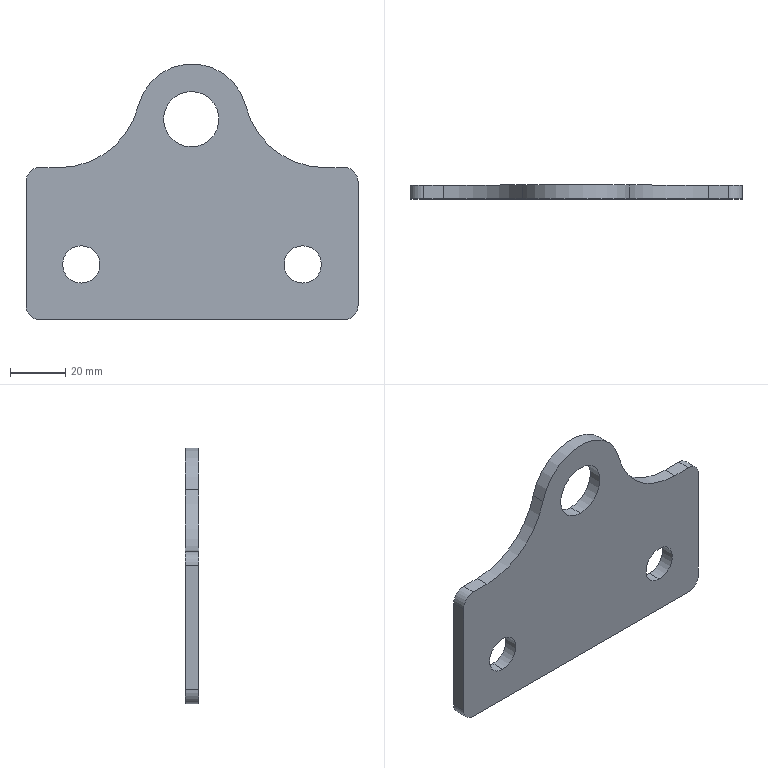Part | 1 solid | 20 faces | box 120 x 5 x 92.5 mm | volume 38056 mm3 | cylinder 13 | plane 7 | commonest cylinder face diameters 10 x4 13.5 x4 20 x2 58.94 x2 40 x1
STEP:
#1=CARTESIAN_POINT('',(40.,0.,-23.25));
#2=VERTEX_POINT('',#1);
#3=CARTESIAN_POINT('',(40.,0.,-36.75));
#4=VERTEX_POINT('',#3);
#5=CARTESIAN_POINT('',(40.,0.,-30.));
#6=DIRECTION('',(0.,-1.,0.));
#7=DIRECTION('',(0.,0.,-1.));
#8=AXIS2_PLACEMENT_3D('',#5,#6,#7);
#9=CIRCLE('',#8,6.75);
#10=EDGE_CURVE('',#2,#4,#9,.T.);
#11=ORIENTED_EDGE('',*,*,#10,.F.);
#12=CARTESIAN_POINT('',(40.,-5.,-23.25));
#13=VERTEX_POINT('',#12);
#14=CARTESIAN_POINT('',(40.,-5.,-23.25));
#15=DIRECTION('',(0.,-1.,0.));
#16=VECTOR('',#15,1000.);
#17=LINE('',#14,#16);
#18=EDGE_CURVE('',#2,#13,#17,.T.);
#19=ORIENTED_EDGE('',*,*,#18,.T.);
#20=CARTESIAN_POINT('',(40.,-5.,-36.75));
#21=VERTEX_POINT('',#20);
#22=CARTESIAN_POINT('',(40.,-5.,-30.));
#23=DIRECTION('',(0.,-1.,0.));
#24=DIRECTION('',(0.,0.,-1.));
#25=AXIS2_PLACEMENT_3D('',#22,#23,#24);
#26=CIRCLE('',#25,6.75);
#27=EDGE_CURVE('',#13,#21,#26,.T.);
#28=ORIENTED_EDGE('',*,*,#27,.T.);
#29=CARTESIAN_POINT('',(40.,-5.,-36.75));
#30=DIRECTION('',(0.,-1.,0.));
#31=VECTOR('',#30,1000.);
#32=LINE('',#29,#31);
#33=EDGE_CURVE('',#4,#21,#32,.T.);
#34=ORIENTED_EDGE('',*,*,#33,.F.);
#35=EDGE_LOOP('',(#11,#19,#28,#34));
#36=FACE_OUTER_BOUND('',#35,.T.);
#37=CARTESIAN_POINT('',(40.,-5.,-30.));
#38=DIRECTION('',(0.,-1.,0.));
#39=DIRECTION('',(0.,0.,-1.));
#40=AXIS2_PLACEMENT_3D('',#37,#38,#39);
#41=CYLINDRICAL_SURFACE('',#40,6.75);
#42=ADVANCED_FACE('',(#36),#41,.F.);
#43=CARTESIAN_POINT('',(-40.,0.,-23.25));
#44=VERTEX_POINT('',#43);
#45=CARTESIAN_POINT('',(-40.,0.,-36.75));
#46=VERTEX_POINT('',#45);
#47=CARTESIAN_POINT('',(-40.,0.,-30.));
#48=DIRECTION('',(0.,-1.,0.));
#49=DIRECTION('',(0.,0.,-1.));
#50=AXIS2_PLACEMENT_3D('',#47,#48,#49);
#51=CIRCLE('',#50,6.75);
#52=EDGE_CURVE('',#44,#46,#51,.T.);
#53=ORIENTED_EDGE('',*,*,#52,.F.);
#54=CARTESIAN_POINT('',(-40.,-5.,-23.25));
#55=VERTEX_POINT('',#54);
#56=CARTESIAN_POINT('',(-40.,-5.,-23.25));
#57=DIRECTION('',(0.,-1.,0.));
#58=VECTOR('',#57,1000.);
#59=LINE('',#56,#58);
#60=EDGE_CURVE('',#44,#55,#59,.T.);
#61=ORIENTED_EDGE('',*,*,#60,.T.);
#62=CARTESIAN_POINT('',(-40.,-5.,-36.75));
#63=VERTEX_POINT('',#62);
#64=CARTESIAN_POINT('',(-40.,-5.,-30.));
#65=DIRECTION('',(0.,-1.,0.));
#66=DIRECTION('',(0.,0.,-1.));
#67=AXIS2_PLACEMENT_3D('',#64,#65,#66);
#68=CIRCLE('',#67,6.75);
#69=EDGE_CURVE('',#55,#63,#68,.T.);
#70=ORIENTED_EDGE('',*,*,#69,.T.);
#71=CARTESIAN_POINT('',(-40.,-5.,-36.75));
#72=DIRECTION('',(0.,-1.,0.));
#73=VECTOR('',#72,1000.);
#74=LINE('',#71,#73);
#75=EDGE_CURVE('',#46,#63,#74,.T.);
#76=ORIENTED_EDGE('',*,*,#75,.F.);
#77=EDGE_LOOP('',(#53,#61,#70,#76));
#78=FACE_OUTER_BOUND('',#77,.T.);
#79=CARTESIAN_POINT('',(-40.,-5.,-30.));
#80=DIRECTION('',(0.,-1.,0.));
#81=DIRECTION('',(0.,0.,-1.));
#82=AXIS2_PLACEMENT_3D('',#79,#80,#81);
#83=CYLINDRICAL_SURFACE('',#82,6.75);
#84=ADVANCED_FACE('',(#78),#83,.F.);
#85=CARTESIAN_POINT('',(-0.25,-5.,32.5));
#86=VERTEX_POINT('',#85);
#87=CARTESIAN_POINT('',(-0.25,-5.,12.5));
#88=VERTEX_POINT('',#87);
#89=CARTESIAN_POINT('',(-0.25,-5.,22.5));
#90=DIRECTION('',(0.,-1.,0.));
#91=DIRECTION('',(0.,0.,-1.));
#92=AXIS2_PLACEMENT_3D('',#89,#90,#91);
#93=CIRCLE('',#92,10.);
#94=EDGE_CURVE('',#86,#88,#93,.T.);
#95=ORIENTED_EDGE('',*,*,#94,.T.);
#96=CARTESIAN_POINT('',(-0.25,0.,12.5));
#97=VERTEX_POINT('',#96);
#98=CARTESIAN_POINT('',(-0.25,-10.,12.5));
#99=DIRECTION('',(0.,1.,0.));
#100=VECTOR('',#99,1000.);
#101=LINE('',#98,#100);
#102=EDGE_CURVE('',#88,#97,#101,.T.);
#103=ORIENTED_EDGE('',*,*,#102,.T.);
#104=CARTESIAN_POINT('',(-0.25,0.,32.5));
#105=VERTEX_POINT('',#104);
#106=CARTESIAN_POINT('',(-0.25,0.,22.5));
#107=DIRECTION('',(0.,1.,0.));
#108=DIRECTION('',(0.,0.,1.));
#109=AXIS2_PLACEMENT_3D('',#106,#107,#108);
#110=CIRCLE('',#109,10.);
#111=EDGE_CURVE('',#97,#105,#110,.T.);
#112=ORIENTED_EDGE('',*,*,#111,.T.);
#113=CARTESIAN_POINT('',(-0.25,-10.,32.5));
#114=DIRECTION('',(0.,1.,0.));
#115=VECTOR('',#114,1000.);
#116=LINE('',#113,#115);
#117=EDGE_CURVE('',#86,#105,#116,.T.);
#118=ORIENTED_EDGE('',*,*,#117,.F.);
#119=EDGE_LOOP('',(#95,#103,#112,#118));
#120=FACE_OUTER_BOUND('',#119,.T.);
#121=CARTESIAN_POINT('',(-0.25,-10.,22.5));
#122=DIRECTION('',(0.,1.,0.));
#123=DIRECTION('',(0.,0.,1.));
#124=AXIS2_PLACEMENT_3D('',#121,#122,#123);
#125=CYLINDRICAL_SURFACE('',#124,10.);
#126=ADVANCED_FACE('',(#120),#125,.F.);
#127=CARTESIAN_POINT('',(40.,-5.,-30.));
#128=DIRECTION('',(0.,-1.,0.));
#129=DIRECTION('',(0.,0.,-1.));
#130=AXIS2_PLACEMENT_3D('',#127,#128,#129);
#131=CIRCLE('',#130,6.75);
#132=EDGE_CURVE('',#21,#13,#131,.T.);
#133=ORIENTED_EDGE('',*,*,#132,.F.);
#134=ORIENTED_EDGE('',*,*,#27,.F.);
#135=EDGE_LOOP('',(#133,#134));
#136=FACE_BOUND('',#135,.T.);
#137=CARTESIAN_POINT('',(-40.,-5.,-30.));
#138=DIRECTION('',(0.,-1.,0.));
#139=DIRECTION('',(0.,0.,-1.));
#140=AXIS2_PLACEMENT_3D('',#137,#138,#139);
#141=CIRCLE('',#140,6.75);
#142=EDGE_CURVE('',#63,#55,#141,.T.);
#143=ORIENTED_EDGE('',*,*,#142,.F.);
#144=ORIENTED_EDGE('',*,*,#69,.F.);
#145=EDGE_LOOP('',(#143,#144));
#146=FACE_BOUND('',#145,.T.);
#147=ORIENTED_EDGE('',*,*,#94,.F.);
#148=CARTESIAN_POINT('',(-0.25,-5.,22.5));
#149=DIRECTION('',(0.,-1.,0.));
#150=DIRECTION('',(0.,0.,-1.));
#151=AXIS2_PLACEMENT_3D('',#148,#149,#150);
#152=CIRCLE('',#151,10.);
#153=EDGE_CURVE('',#88,#86,#152,.T.);
#154=ORIENTED_EDGE('',*,*,#153,.F.);
#155=EDGE_LOOP('',(#147,#154));
#156=FACE_BOUND('',#155,.T.);
#157=CARTESIAN_POINT('',(-60.,-5.,-45.));
#158=VERTEX_POINT('',#157);
#159=CARTESIAN_POINT('',(-60.,-5.,0.));
#160=VERTEX_POINT('',#159);
#161=CARTESIAN_POINT('',(-60.,-5.,50.));
#162=DIRECTION('',(0.,0.,1.));
#163=VECTOR('',#162,1000.);
#164=LINE('',#161,#163);
#165=EDGE_CURVE('',#158,#160,#164,.T.);
#166=ORIENTED_EDGE('',*,*,#165,.F.);
#167=CARTESIAN_POINT('',(-55.,-5.,-50.));
#168=VERTEX_POINT('',#167);
#169=CARTESIAN_POINT('',(-55.,-5.,-45.));
#170=DIRECTION('',(0.,-1.,0.));
#171=DIRECTION('',(0.,0.,-1.));
#172=AXIS2_PLACEMENT_3D('',#169,#170,#171);
#173=CIRCLE('',#172,5.);
#174=EDGE_CURVE('',#158,#168,#173,.T.);
#175=ORIENTED_EDGE('',*,*,#174,.T.);
#176=CARTESIAN_POINT('',(55.,-5.,-50.));
#177=VERTEX_POINT('',#176);
#178=CARTESIAN_POINT('',(-60.,-5.,-50.));
#179=DIRECTION('',(-1.,0.,0.));
#180=VECTOR('',#179,1000.);
#181=LINE('',#178,#180);
#182=EDGE_CURVE('',#177,#168,#181,.T.);
#183=ORIENTED_EDGE('',*,*,#182,.F.);
#184=CARTESIAN_POINT('',(60.,-5.,-45.));
#185=VERTEX_POINT('',#184);
#186=CARTESIAN_POINT('',(55.,-5.,-45.));
#187=DIRECTION('',(0.,-1.,0.));
#188=DIRECTION('',(0.,0.,-1.));
#189=AXIS2_PLACEMENT_3D('',#186,#187,#188);
#190=CIRCLE('',#189,5.);
#191=EDGE_CURVE('',#177,#185,#190,.T.);
#192=ORIENTED_EDGE('',*,*,#191,.T.);
#193=CARTESIAN_POINT('',(60.,-5.,0.));
#194=VERTEX_POINT('',#193);
#195=CARTESIAN_POINT('',(60.,-5.,50.));
#196=DIRECTION('',(0.,0.,-1.));
#197=VECTOR('',#196,1000.);
#198=LINE('',#195,#197);
#199=EDGE_CURVE('',#194,#185,#198,.T.);
#200=ORIENTED_EDGE('',*,*,#199,.F.);
#201=CARTESIAN_POINT('',(55.,-5.,5.));
#202=VERTEX_POINT('',#201);
#203=CARTESIAN_POINT('',(55.,-5.,0.));
#204=DIRECTION('',(0.,-1.,0.));
#205=DIRECTION('',(0.,0.,-1.));
#206=AXIS2_PLACEMENT_3D('',#203,#204,#205);
#207=CIRCLE('',#206,5.);
#208=EDGE_CURVE('',#194,#202,#207,.T.);
#209=ORIENTED_EDGE('',*,*,#208,.T.);
#210=CARTESIAN_POINT('',(48.,-5.,5.));
#211=VERTEX_POINT('',#210);
#212=CARTESIAN_POINT('',(60.,-5.,5.));
#213=DIRECTION('',(1.,0.,0.));
#214=VECTOR('',#213,1000.);
#215=LINE('',#212,#214);
#216=EDGE_CURVE('',#211,#202,#215,.T.);
#217=ORIENTED_EDGE('',*,*,#216,.F.);
#218=CARTESIAN_POINT('',(19.406,-5.,27.339));
#219=VERTEX_POINT('',#218);
#220=CARTESIAN_POINT('',(48.,-5.,34.47));
#221=DIRECTION('',(0.,-1.,0.));
#222=DIRECTION('',(0.,0.,-1.));
#223=AXIS2_PLACEMENT_3D('',#220,#221,#222);
#224=CIRCLE('',#223,29.47);
#225=EDGE_CURVE('',#219,#211,#224,.T.);
#226=ORIENTED_EDGE('',*,*,#225,.F.);
#227=CARTESIAN_POINT('',(-19.406,-5.,27.339));
#228=VERTEX_POINT('',#227);
#229=CARTESIAN_POINT('',(0.,-5.,22.5));
#230=DIRECTION('',(0.,1.,0.));
#231=DIRECTION('',(0.,0.,-1.));
#232=AXIS2_PLACEMENT_3D('',#229,#230,#231);
#233=CIRCLE('',#232,20.);
#234=EDGE_CURVE('',#228,#219,#233,.T.);
#235=ORIENTED_EDGE('',*,*,#234,.F.);
#236=CARTESIAN_POINT('',(-48.,-5.,5.));
#237=VERTEX_POINT('',#236);
#238=CARTESIAN_POINT('',(-48.,-5.,34.47));
#239=DIRECTION('',(0.,-1.,0.));
#240=DIRECTION('',(0.,0.,1.));
#241=AXIS2_PLACEMENT_3D('',#238,#239,#240);
#242=CIRCLE('',#241,29.47);
#243=EDGE_CURVE('',#237,#228,#242,.T.);
#244=ORIENTED_EDGE('',*,*,#243,.F.);
#245=CARTESIAN_POINT('',(-55.,-5.,5.));
#246=VERTEX_POINT('',#245);
#247=CARTESIAN_POINT('',(-48.,-5.,5.));
#248=DIRECTION('',(1.,0.,0.));
#249=VECTOR('',#248,1000.);
#250=LINE('',#247,#249);
#251=EDGE_CURVE('',#246,#237,#250,.T.);
#252=ORIENTED_EDGE('',*,*,#251,.F.);
#253=CARTESIAN_POINT('',(-55.,-5.,0.));
#254=DIRECTION('',(0.,-1.,0.));
#255=DIRECTION('',(0.,0.,-1.));
#256=AXIS2_PLACEMENT_3D('',#253,#254,#255);
#257=CIRCLE('',#256,5.);
#258=EDGE_CURVE('',#246,#160,#257,.T.);
#259=ORIENTED_EDGE('',*,*,#258,.T.);
#260=EDGE_LOOP('',(#166,#175,#183,#192,#200,#209,#217,#226,#235,#244,#252,#259));
#261=FACE_OUTER_BOUND('',#260,.T.);
#262=CARTESIAN_POINT('',(0.,-5.,0.));
#263=DIRECTION('',(0.,-1.,0.));
#264=DIRECTION('',(0.,0.,-1.));
#265=AXIS2_PLACEMENT_3D('',#262,#263,#264);
#266=PLANE('',#265);
#267=ADVANCED_FACE('',(#136,#146,#156,#261),#266,.T.);
#268=CARTESIAN_POINT('',(40.,0.,-30.));
#269=DIRECTION('',(0.,-1.,0.));
#270=DIRECTION('',(0.,0.,-1.));
#271=AXIS2_PLACEMENT_3D('',#268,#269,#270);
#272=CIRCLE('',#271,6.75);
#273=EDGE_CURVE('',#4,#2,#272,.T.);
#274=ORIENTED_EDGE('',*,*,#273,.T.);
#275=ORIENTED_EDGE('',*,*,#10,.T.);
#276=EDGE_LOOP('',(#274,#275));
#277=FACE_BOUND('',#276,.T.);
#278=CARTESIAN_POINT('',(-40.,0.,-30.));
#279=DIRECTION('',(0.,-1.,0.));
#280=DIRECTION('',(0.,0.,-1.));
#281=AXIS2_PLACEMENT_3D('',#278,#279,#280);
#282=CIRCLE('',#281,6.75);
#283=EDGE_CURVE('',#46,#44,#282,.T.);
#284=ORIENTED_EDGE('',*,*,#283,.T.);
#285=ORIENTED_EDGE('',*,*,#52,.T.);
#286=EDGE_LOOP('',(#284,#285));
#287=FACE_BOUND('',#286,.T.);
#288=CARTESIAN_POINT('',(-0.25,0.,22.5));
#289=DIRECTION('',(0.,1.,0.));
#290=DIRECTION('',(0.,0.,1.));
#291=AXIS2_PLACEMENT_3D('',#288,#289,#290);
#292=CIRCLE('',#291,10.);
#293=EDGE_CURVE('',#105,#97,#292,.T.);
#294=ORIENTED_EDGE('',*,*,#293,.F.);
#295=ORIENTED_EDGE('',*,*,#111,.F.);
#296=EDGE_LOOP('',(#294,#295));
#297=FACE_BOUND('',#296,.T.);
#298=CARTESIAN_POINT('',(55.,0.,-50.));
#299=VERTEX_POINT('',#298);
#300=CARTESIAN_POINT('',(-55.,0.,-50.));
#301=VERTEX_POINT('',#300);
#302=CARTESIAN_POINT('',(-60.,0.,-50.));
#303=DIRECTION('',(-1.,0.,0.));
#304=VECTOR('',#303,1000.);
#305=LINE('',#302,#304);
#306=EDGE_CURVE('',#299,#301,#305,.T.);
#307=ORIENTED_EDGE('',*,*,#306,.T.);
#308=CARTESIAN_POINT('',(-60.,0.,-45.));
#309=VERTEX_POINT('',#308);
#310=CARTESIAN_POINT('',(-55.,0.,-45.));
#311=DIRECTION('',(0.,1.,0.));
#312=DIRECTION('',(0.,0.,-1.));
#313=AXIS2_PLACEMENT_3D('',#310,#311,#312);
#314=CIRCLE('',#313,5.);
#315=EDGE_CURVE('',#301,#309,#314,.T.);
#316=ORIENTED_EDGE('',*,*,#315,.T.);
#317=CARTESIAN_POINT('',(-60.,0.,0.));
#318=VERTEX_POINT('',#317);
#319=CARTESIAN_POINT('',(-60.,0.,50.));
#320=DIRECTION('',(0.,0.,1.));
#321=VECTOR('',#320,1000.);
#322=LINE('',#319,#321);
#323=EDGE_CURVE('',#309,#318,#322,.T.);
#324=ORIENTED_EDGE('',*,*,#323,.T.);
#325=CARTESIAN_POINT('',(-55.,0.,5.));
#326=VERTEX_POINT('',#325);
#327=CARTESIAN_POINT('',(-55.,0.,0.));
#328=DIRECTION('',(0.,1.,0.));
#329=DIRECTION('',(0.,0.,-1.));
#330=AXIS2_PLACEMENT_3D('',#327,#328,#329);
#331=CIRCLE('',#330,5.);
#332=EDGE_CURVE('',#318,#326,#331,.T.);
#333=ORIENTED_EDGE('',*,*,#332,.T.);
#334=CARTESIAN_POINT('',(-48.,0.,5.));
#335=VERTEX_POINT('',#334);
#336=CARTESIAN_POINT('',(-48.,0.,5.));
#337=DIRECTION('',(1.,0.,0.));
#338=VECTOR('',#337,1000.);
#339=LINE('',#336,#338);
#340=EDGE_CURVE('',#326,#335,#339,.T.);
#341=ORIENTED_EDGE('',*,*,#340,.T.);
#342=CARTESIAN_POINT('',(-19.406,0.,27.339));
#343=VERTEX_POINT('',#342);
#344=CARTESIAN_POINT('',(-48.,0.,34.47));
#345=DIRECTION('',(0.,-1.,0.));
#346=DIRECTION('',(0.,0.,1.));
#347=AXIS2_PLACEMENT_3D('',#344,#345,#346);
#348=CIRCLE('',#347,29.47);
#349=EDGE_CURVE('',#335,#343,#348,.T.);
#350=ORIENTED_EDGE('',*,*,#349,.T.);
#351=CARTESIAN_POINT('',(19.406,0.,27.339));
#352=VERTEX_POINT('',#351);
#353=CARTESIAN_POINT('',(0.,0.,22.5));
#354=DIRECTION('',(0.,1.,0.));
#355=DIRECTION('',(0.,0.,-1.));
#356=AXIS2_PLACEMENT_3D('',#353,#354,#355);
#357=CIRCLE('',#356,20.);
#358=EDGE_CURVE('',#343,#352,#357,.T.);
#359=ORIENTED_EDGE('',*,*,#358,.T.);
#360=CARTESIAN_POINT('',(48.,0.,5.));
#361=VERTEX_POINT('',#360);
#362=CARTESIAN_POINT('',(48.,0.,34.47));
#363=DIRECTION('',(0.,-1.,0.));
#364=DIRECTION('',(0.,0.,-1.));
#365=AXIS2_PLACEMENT_3D('',#362,#363,#364);
#366=CIRCLE('',#365,29.47);
#367=EDGE_CURVE('',#352,#361,#366,.T.);
#368=ORIENTED_EDGE('',*,*,#367,.T.);
#369=CARTESIAN_POINT('',(55.,0.,5.));
#370=VERTEX_POINT('',#369);
#371=CARTESIAN_POINT('',(60.,0.,5.));
#372=DIRECTION('',(1.,0.,0.));
#373=VECTOR('',#372,1000.);
#374=LINE('',#371,#373);
#375=EDGE_CURVE('',#361,#370,#374,.T.);
#376=ORIENTED_EDGE('',*,*,#375,.T.);
#377=CARTESIAN_POINT('',(60.,0.,0.));
#378=VERTEX_POINT('',#377);
#379=CARTESIAN_POINT('',(55.,0.,0.));
#380=DIRECTION('',(0.,1.,0.));
#381=DIRECTION('',(0.,0.,-1.));
#382=AXIS2_PLACEMENT_3D('',#379,#380,#381);
#383=CIRCLE('',#382,5.);
#384=EDGE_CURVE('',#370,#378,#383,.T.);
#385=ORIENTED_EDGE('',*,*,#384,.T.);
#386=CARTESIAN_POINT('',(60.,0.,-45.));
#387=VERTEX_POINT('',#386);
#388=CARTESIAN_POINT('',(60.,0.,50.));
#389=DIRECTION('',(0.,0.,-1.));
#390=VECTOR('',#389,1000.);
#391=LINE('',#388,#390);
#392=EDGE_CURVE('',#378,#387,#391,.T.);
#393=ORIENTED_EDGE('',*,*,#392,.T.);
#394=CARTESIAN_POINT('',(55.,0.,-45.));
#395=DIRECTION('',(0.,1.,0.));
#396=DIRECTION('',(0.,0.,-1.));
#397=AXIS2_PLACEMENT_3D('',#394,#395,#396);
#398=CIRCLE('',#397,5.);
#399=EDGE_CURVE('',#387,#299,#398,.T.);
#400=ORIENTED_EDGE('',*,*,#399,.T.);
#401=EDGE_LOOP('',(#307,#316,#324,#333,#341,#350,#359,#368,#376,#385,#393,#400));
#402=FACE_OUTER_BOUND('',#401,.T.);
#403=CARTESIAN_POINT('',(0.,0.,0.));
#404=DIRECTION('',(0.,-1.,0.));
#405=DIRECTION('',(0.,0.,-1.));
#406=AXIS2_PLACEMENT_3D('',#403,#404,#405);
#407=PLANE('',#406);
#408=ADVANCED_FACE('',(#277,#287,#297,#402),#407,.F.);
#409=ORIENTED_EDGE('',*,*,#199,.T.);
#410=CARTESIAN_POINT('',(60.,-5.,-45.));
#411=DIRECTION('',(0.,1.,0.));
#412=VECTOR('',#411,1000.);
#413=LINE('',#410,#412);
#414=EDGE_CURVE('',#185,#387,#413,.T.);
#415=ORIENTED_EDGE('',*,*,#414,.T.);
#416=ORIENTED_EDGE('',*,*,#392,.F.);
#417=CARTESIAN_POINT('',(60.,-5.,0.));
#418=DIRECTION('',(0.,-1.,0.));
#419=VECTOR('',#418,1000.);
#420=LINE('',#417,#419);
#421=EDGE_CURVE('',#378,#194,#420,.T.);
#422=ORIENTED_EDGE('',*,*,#421,.T.);
#423=EDGE_LOOP('',(#409,#415,#416,#422));
#424=FACE_OUTER_BOUND('',#423,.T.);
#425=CARTESIAN_POINT('',(60.,-5.,50.));
#426=DIRECTION('',(1.,0.,0.));
#427=DIRECTION('',(0.,0.,-1.));
#428=AXIS2_PLACEMENT_3D('',#425,#426,#427);
#429=PLANE('',#428);
#430=ADVANCED_FACE('',(#424),#429,.T.);
#431=ORIENTED_EDGE('',*,*,#323,.F.);
#432=CARTESIAN_POINT('',(-60.,-5.,-45.));
#433=DIRECTION('',(0.,-1.,0.));
#434=VECTOR('',#433,1000.);
#435=LINE('',#432,#434);
#436=EDGE_CURVE('',#309,#158,#435,.T.);
#437=ORIENTED_EDGE('',*,*,#436,.T.);
#438=ORIENTED_EDGE('',*,*,#165,.T.);
#439=CARTESIAN_POINT('',(-60.,0.,0.));
#440=DIRECTION('',(0.,1.,0.));
#441=VECTOR('',#440,1000.);
#442=LINE('',#439,#441);
#443=EDGE_CURVE('',#160,#318,#442,.T.);
#444=ORIENTED_EDGE('',*,*,#443,.T.);
#445=EDGE_LOOP('',(#431,#437,#438,#444));
#446=FACE_OUTER_BOUND('',#445,.T.);
#447=CARTESIAN_POINT('',(-60.,-5.,50.));
#448=DIRECTION('',(-1.,0.,0.));
#449=DIRECTION('',(0.,0.,1.));
#450=AXIS2_PLACEMENT_3D('',#447,#448,#449);
#451=PLANE('',#450);
#452=ADVANCED_FACE('',(#446),#451,.T.);
#453=ORIENTED_EDGE('',*,*,#182,.T.);
#454=CARTESIAN_POINT('',(-55.,-5.,-50.));
#455=DIRECTION('',(0.,1.,0.));
#456=VECTOR('',#455,1000.);
#457=LINE('',#454,#456);
#458=EDGE_CURVE('',#168,#301,#457,.T.);
#459=ORIENTED_EDGE('',*,*,#458,.T.);
#460=ORIENTED_EDGE('',*,*,#306,.F.);
#461=CARTESIAN_POINT('',(55.,-5.,-50.));
#462=DIRECTION('',(0.,-1.,0.));
#463=VECTOR('',#462,1000.);
#464=LINE('',#461,#463);
#465=EDGE_CURVE('',#299,#177,#464,.T.);
#466=ORIENTED_EDGE('',*,*,#465,.T.);
#467=EDGE_LOOP('',(#453,#459,#460,#466));
#468=FACE_OUTER_BOUND('',#467,.T.);
#469=CARTESIAN_POINT('',(-60.,-5.,-50.));
#470=DIRECTION('',(0.,0.,-1.));
#471=DIRECTION('',(-1.,0.,0.));
#472=AXIS2_PLACEMENT_3D('',#469,#470,#471);
#473=PLANE('',#472);
#474=ADVANCED_FACE('',(#468),#473,.T.);
#475=ORIENTED_EDGE('',*,*,#102,.F.);
#476=ORIENTED_EDGE('',*,*,#153,.T.);
#477=ORIENTED_EDGE('',*,*,#117,.T.);
#478=ORIENTED_EDGE('',*,*,#293,.T.);
#479=EDGE_LOOP('',(#475,#476,#477,#478));
#480=FACE_OUTER_BOUND('',#479,.T.);
#481=CARTESIAN_POINT('',(-0.25,-10.,22.5));
#482=DIRECTION('',(0.,1.,0.));
#483=DIRECTION('',(0.,0.,1.));
#484=AXIS2_PLACEMENT_3D('',#481,#482,#483);
#485=CYLINDRICAL_SURFACE('',#484,10.);
#486=ADVANCED_FACE('',(#480),#485,.F.);
#487=ORIENTED_EDGE('',*,*,#243,.T.);
#488=CARTESIAN_POINT('',(-19.406,0.,27.339));
#489=DIRECTION('',(0.,-1.,0.));
#490=VECTOR('',#489,1000.);
#491=LINE('',#488,#490);
#492=EDGE_CURVE('',#343,#228,#491,.T.);
#493=ORIENTED_EDGE('',*,*,#492,.F.);
#494=ORIENTED_EDGE('',*,*,#349,.F.);
#495=CARTESIAN_POINT('',(-48.,0.,5.));
#496=DIRECTION('',(0.,-1.,0.));
#497=VECTOR('',#496,1000.);
#498=LINE('',#495,#497);
#499=EDGE_CURVE('',#335,#237,#498,.T.);
#500=ORIENTED_EDGE('',*,*,#499,.T.);
#501=EDGE_LOOP('',(#487,#493,#494,#500));
#502=FACE_OUTER_BOUND('',#501,.T.);
#503=CARTESIAN_POINT('',(-48.,0.,34.47));
#504=DIRECTION('',(0.,-1.,0.));
#505=DIRECTION('',(0.,0.,-1.));
#506=AXIS2_PLACEMENT_3D('',#503,#504,#505);
#507=CYLINDRICAL_SURFACE('',#506,29.47);
#508=ADVANCED_FACE('',(#502),#507,.F.);
#509=ORIENTED_EDGE('',*,*,#340,.F.);
#510=CARTESIAN_POINT('',(-55.,-5.,5.));
#511=DIRECTION('',(0.,-1.,0.));
#512=VECTOR('',#511,1000.);
#513=LINE('',#510,#512);
#514=EDGE_CURVE('',#326,#246,#513,.T.);
#515=ORIENTED_EDGE('',*,*,#514,.T.);
#516=ORIENTED_EDGE('',*,*,#251,.T.);
#517=ORIENTED_EDGE('',*,*,#499,.F.);
#518=EDGE_LOOP('',(#509,#515,#516,#517));
#519=FACE_OUTER_BOUND('',#518,.T.);
#520=CARTESIAN_POINT('',(-48.,0.,5.));
#521=DIRECTION('',(0.,0.,-1.));
#522=DIRECTION('',(-1.,0.,0.));
#523=AXIS2_PLACEMENT_3D('',#520,#521,#522);
#524=PLANE('',#523);
#525=ADVANCED_FACE('',(#519),#524,.F.);
#526=ORIENTED_EDGE('',*,*,#216,.T.);
#527=CARTESIAN_POINT('',(55.,0.,5.));
#528=DIRECTION('',(0.,1.,0.));
#529=VECTOR('',#528,1000.);
#530=LINE('',#527,#529);
#531=EDGE_CURVE('',#202,#370,#530,.T.);
#532=ORIENTED_EDGE('',*,*,#531,.T.);
#533=ORIENTED_EDGE('',*,*,#375,.F.);
#534=CARTESIAN_POINT('',(48.,0.,5.));
#535=DIRECTION('',(0.,-1.,0.));
#536=VECTOR('',#535,1000.);
#537=LINE('',#534,#536);
#538=EDGE_CURVE('',#361,#211,#537,.T.);
#539=ORIENTED_EDGE('',*,*,#538,.T.);
#540=EDGE_LOOP('',(#526,#532,#533,#539));
#541=FACE_OUTER_BOUND('',#540,.T.);
#542=CARTESIAN_POINT('',(60.,0.,5.));
#543=DIRECTION('',(0.,0.,-1.));
#544=DIRECTION('',(-1.,0.,0.));
#545=AXIS2_PLACEMENT_3D('',#542,#543,#544);
#546=PLANE('',#545);
#547=ADVANCED_FACE('',(#541),#546,.F.);
#548=ORIENTED_EDGE('',*,*,#225,.T.);
#549=ORIENTED_EDGE('',*,*,#538,.F.);
#550=ORIENTED_EDGE('',*,*,#367,.F.);
#551=CARTESIAN_POINT('',(19.406,0.,27.339));
#552=DIRECTION('',(0.,-1.,0.));
#553=VECTOR('',#552,1000.);
#554=LINE('',#551,#553);
#555=EDGE_CURVE('',#352,#219,#554,.T.);
#556=ORIENTED_EDGE('',*,*,#555,.T.);
#557=EDGE_LOOP('',(#548,#549,#550,#556));
#558=FACE_OUTER_BOUND('',#557,.T.);
#559=CARTESIAN_POINT('',(48.,0.,34.47));
#560=DIRECTION('',(0.,-1.,0.));
#561=DIRECTION('',(0.,0.,-1.));
#562=AXIS2_PLACEMENT_3D('',#559,#560,#561);
#563=CYLINDRICAL_SURFACE('',#562,29.47);
#564=ADVANCED_FACE('',(#558),#563,.F.);
#565=ORIENTED_EDGE('',*,*,#234,.T.);
#566=ORIENTED_EDGE('',*,*,#555,.F.);
#567=ORIENTED_EDGE('',*,*,#358,.F.);
#568=ORIENTED_EDGE('',*,*,#492,.T.);
#569=EDGE_LOOP('',(#565,#566,#567,#568));
#570=FACE_OUTER_BOUND('',#569,.T.);
#571=CARTESIAN_POINT('',(0.,0.,22.5));
#572=DIRECTION('',(0.,-1.,0.));
#573=DIRECTION('',(0.,0.,-1.));
#574=AXIS2_PLACEMENT_3D('',#571,#572,#573);
#575=CYLINDRICAL_SURFACE('',#574,20.);
#576=ADVANCED_FACE('',(#570),#575,.T.);
#577=ORIENTED_EDGE('',*,*,#174,.F.);
#578=ORIENTED_EDGE('',*,*,#436,.F.);
#579=ORIENTED_EDGE('',*,*,#315,.F.);
#580=ORIENTED_EDGE('',*,*,#458,.F.);
#581=EDGE_LOOP('',(#577,#578,#579,#580));
#582=FACE_OUTER_BOUND('',#581,.T.);
#583=CARTESIAN_POINT('',(-55.,-5.,-45.));
#584=DIRECTION('',(0.,1.,0.));
#585=DIRECTION('',(0.,0.,1.));
#586=AXIS2_PLACEMENT_3D('',#583,#584,#585);
#587=CYLINDRICAL_SURFACE('',#586,5.);
#588=ADVANCED_FACE('',(#582),#587,.T.);
#589=ORIENTED_EDGE('',*,*,#332,.F.);
#590=ORIENTED_EDGE('',*,*,#443,.F.);
#591=ORIENTED_EDGE('',*,*,#258,.F.);
#592=ORIENTED_EDGE('',*,*,#514,.F.);
#593=EDGE_LOOP('',(#589,#590,#591,#592));
#594=FACE_OUTER_BOUND('',#593,.T.);
#595=CARTESIAN_POINT('',(-55.,0.,0.));
#596=DIRECTION('',(0.,1.,0.));
#597=DIRECTION('',(0.,0.,1.));
#598=AXIS2_PLACEMENT_3D('',#595,#596,#597);
#599=CYLINDRICAL_SURFACE('',#598,5.);
#600=ADVANCED_FACE('',(#594),#599,.T.);
#601=ORIENTED_EDGE('',*,*,#191,.F.);
#602=ORIENTED_EDGE('',*,*,#465,.F.);
#603=ORIENTED_EDGE('',*,*,#399,.F.);
#604=ORIENTED_EDGE('',*,*,#414,.F.);
#605=EDGE_LOOP('',(#601,#602,#603,#604));
#606=FACE_OUTER_BOUND('',#605,.T.);
#607=CARTESIAN_POINT('',(55.,-5.,-45.));
#608=DIRECTION('',(0.,1.,0.));
#609=DIRECTION('',(0.,0.,1.));
#610=AXIS2_PLACEMENT_3D('',#607,#608,#609);
#611=CYLINDRICAL_SURFACE('',#610,5.);
#612=ADVANCED_FACE('',(#606),#611,.T.);
#613=ORIENTED_EDGE('',*,*,#384,.F.);
#614=ORIENTED_EDGE('',*,*,#531,.F.);
#615=ORIENTED_EDGE('',*,*,#208,.F.);
#616=ORIENTED_EDGE('',*,*,#421,.F.);
#617=EDGE_LOOP('',(#613,#614,#615,#616));
#618=FACE_OUTER_BOUND('',#617,.T.);
#619=CARTESIAN_POINT('',(55.,-5.,0.));
#620=DIRECTION('',(0.,1.,0.));
#621=DIRECTION('',(0.,0.,1.));
#622=AXIS2_PLACEMENT_3D('',#619,#620,#621);
#623=CYLINDRICAL_SURFACE('',#622,5.);
#624=ADVANCED_FACE('',(#618),#623,.T.);
#625=ORIENTED_EDGE('',*,*,#60,.F.);
#626=ORIENTED_EDGE('',*,*,#283,.F.);
#627=ORIENTED_EDGE('',*,*,#75,.T.);
#628=ORIENTED_EDGE('',*,*,#142,.T.);
#629=EDGE_LOOP('',(#625,#626,#627,#628));
#630=FACE_OUTER_BOUND('',#629,.T.);
#631=CARTESIAN_POINT('',(-40.,-5.,-30.));
#632=DIRECTION('',(0.,-1.,0.));
#633=DIRECTION('',(0.,0.,-1.));
#634=AXIS2_PLACEMENT_3D('',#631,#632,#633);
#635=CYLINDRICAL_SURFACE('',#634,6.75);
#636=ADVANCED_FACE('',(#630),#635,.F.);
#637=ORIENTED_EDGE('',*,*,#18,.F.);
#638=ORIENTED_EDGE('',*,*,#273,.F.);
#639=ORIENTED_EDGE('',*,*,#33,.T.);
#640=ORIENTED_EDGE('',*,*,#132,.T.);
#641=EDGE_LOOP('',(#637,#638,#639,#640));
#642=FACE_OUTER_BOUND('',#641,.T.);
#643=CARTESIAN_POINT('',(40.,-5.,-30.));
#644=DIRECTION('',(0.,-1.,0.));
#645=DIRECTION('',(0.,0.,-1.));
#646=AXIS2_PLACEMENT_3D('',#643,#644,#645);
#647=CYLINDRICAL_SURFACE('',#646,6.75);
#648=ADVANCED_FACE('',(#642),#647,.F.);
#649=CLOSED_SHELL('',(#42,#84,#126,#267,#408,#430,#452,#474,#486,#508,#525,#547,#564,#576,#588,#600,#612,#624,#636,#648));
#650=MANIFOLD_SOLID_BREP('',#649);
#651=CARTESIAN_POINT('',(0.,0.,0.));
#652=DIRECTION('',(0.,0.,1.));
#653=DIRECTION('',(1.,0.,0.));
#654=AXIS2_PLACEMENT_3D('',#651,#652,#653);
#655=(LENGTH_UNIT()NAMED_UNIT(*)SI_UNIT(.MILLI.,.METRE.));
#656=UNCERTAINTY_MEASURE_WITH_UNIT(LENGTH_MEASURE(0.00001),#655,'','');
#657=(NAMED_UNIT(*)PLANE_ANGLE_UNIT()SI_UNIT($,.RADIAN.));
#658=(NAMED_UNIT(*)SI_UNIT($,.STERADIAN.)SOLID_ANGLE_UNIT());
#659=(GEOMETRIC_REPRESENTATION_CONTEXT(3)GLOBAL_UNCERTAINTY_ASSIGNED_CONTEXT((#656))GLOBAL_UNIT_ASSIGNED_CONTEXT((#655,#657,#658))REPRESENTATION_CONTEXT('',''));
#660=ADVANCED_BREP_SHAPE_REPRESENTATION('',(#650,#654),#659);